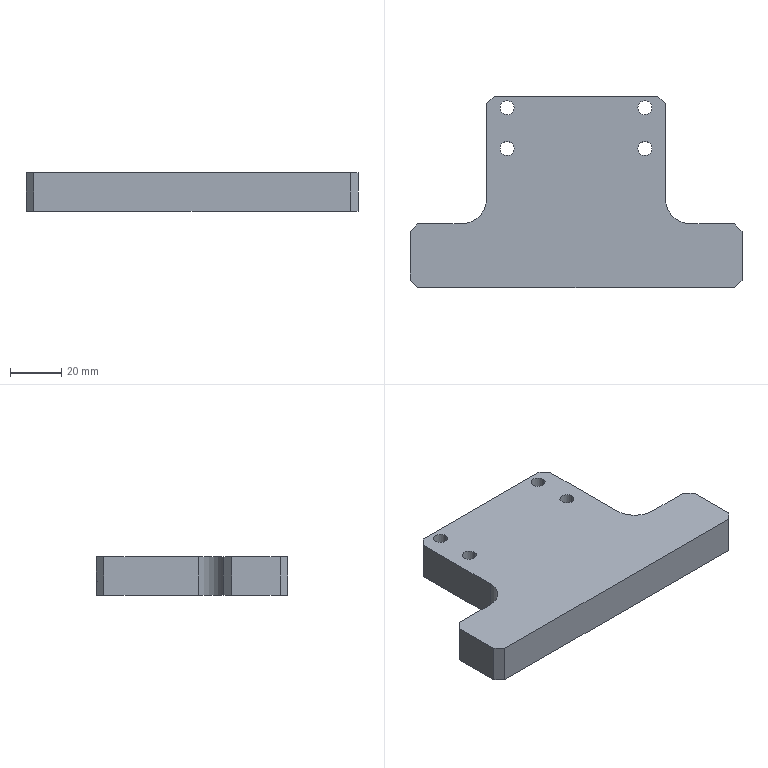Part | SolidWorks | features BaseBody 1 | 1 solid | 40 faces | box 130 x 75 x 15 mm | volume 98795 mm3 | plane 24 | cylinder 16 | commonest cylinder face diameters 5.5 x8 10 x6 20 x2
STEP:
#1=CARTESIAN_POINT('',(29.75,33.,15.));
#2=VERTEX_POINT('',#1);
#3=CARTESIAN_POINT('',(24.25,33.,15.));
#4=VERTEX_POINT('',#3);
#5=CARTESIAN_POINT('',(27.,33.,15.));
#6=DIRECTION('',(0.,0.,-1.));
#7=DIRECTION('',(-1.,0.,0.));
#8=AXIS2_PLACEMENT_3D('',#5,#6,#7);
#9=CIRCLE('',#8,2.75);
#10=EDGE_CURVE('',#2,#4,#9,.T.);
#11=ORIENTED_EDGE('',*,*,#10,.F.);
#12=CARTESIAN_POINT('',(29.75,33.,5.5));
#13=VERTEX_POINT('',#12);
#14=CARTESIAN_POINT('',(29.75,33.,0.));
#15=DIRECTION('',(0.,0.,-1.));
#16=VECTOR('',#15,1000.);
#17=LINE('',#14,#16);
#18=EDGE_CURVE('',#2,#13,#17,.T.);
#19=ORIENTED_EDGE('',*,*,#18,.T.);
#20=CARTESIAN_POINT('',(24.25,33.,5.5));
#21=VERTEX_POINT('',#20);
#22=CARTESIAN_POINT('',(27.,33.,5.5));
#23=DIRECTION('',(0.,0.,-1.));
#24=DIRECTION('',(-1.,0.,0.));
#25=AXIS2_PLACEMENT_3D('',#22,#23,#24);
#26=CIRCLE('',#25,2.75);
#27=EDGE_CURVE('',#13,#21,#26,.T.);
#28=ORIENTED_EDGE('',*,*,#27,.T.);
#29=CARTESIAN_POINT('',(24.25,33.,0.));
#30=DIRECTION('',(0.,0.,-1.));
#31=VECTOR('',#30,1000.);
#32=LINE('',#29,#31);
#33=EDGE_CURVE('',#4,#21,#32,.T.);
#34=ORIENTED_EDGE('',*,*,#33,.F.);
#35=EDGE_LOOP('',(#11,#19,#28,#34));
#36=FACE_OUTER_BOUND('',#35,.T.);
#37=CARTESIAN_POINT('',(27.,33.,0.));
#38=DIRECTION('',(0.,0.,-1.));
#39=DIRECTION('',(-1.,0.,0.));
#40=AXIS2_PLACEMENT_3D('',#37,#38,#39);
#41=CYLINDRICAL_SURFACE('',#40,2.75);
#42=ADVANCED_FACE('',(#36),#41,.F.);
#43=CARTESIAN_POINT('',(32.,17.,5.5));
#44=VERTEX_POINT('',#43);
#45=CARTESIAN_POINT('',(22.,17.,5.5));
#46=VERTEX_POINT('',#45);
#47=CARTESIAN_POINT('',(27.,17.,5.5));
#48=DIRECTION('',(0.,0.,-1.));
#49=DIRECTION('',(-1.,0.,0.));
#50=AXIS2_PLACEMENT_3D('',#47,#48,#49);
#51=CIRCLE('',#50,5.);
#52=EDGE_CURVE('',#44,#46,#51,.T.);
#53=ORIENTED_EDGE('',*,*,#52,.F.);
#54=CARTESIAN_POINT('',(32.,17.,0.));
#55=VERTEX_POINT('',#54);
#56=CARTESIAN_POINT('',(32.,17.,0.));
#57=DIRECTION('',(0.,0.,-1.));
#58=VECTOR('',#57,1000.);
#59=LINE('',#56,#58);
#60=EDGE_CURVE('',#44,#55,#59,.T.);
#61=ORIENTED_EDGE('',*,*,#60,.T.);
#62=CARTESIAN_POINT('',(22.,17.,0.));
#63=VERTEX_POINT('',#62);
#64=CARTESIAN_POINT('',(27.,17.,0.));
#65=DIRECTION('',(0.,0.,-1.));
#66=DIRECTION('',(-1.,0.,0.));
#67=AXIS2_PLACEMENT_3D('',#64,#65,#66);
#68=CIRCLE('',#67,5.);
#69=EDGE_CURVE('',#55,#63,#68,.T.);
#70=ORIENTED_EDGE('',*,*,#69,.T.);
#71=CARTESIAN_POINT('',(22.,17.,0.));
#72=DIRECTION('',(0.,0.,-1.));
#73=VECTOR('',#72,1000.);
#74=LINE('',#71,#73);
#75=EDGE_CURVE('',#46,#63,#74,.T.);
#76=ORIENTED_EDGE('',*,*,#75,.F.);
#77=EDGE_LOOP('',(#53,#61,#70,#76));
#78=FACE_OUTER_BOUND('',#77,.T.);
#79=CARTESIAN_POINT('',(27.,17.,0.));
#80=DIRECTION('',(0.,0.,-1.));
#81=DIRECTION('',(-1.,0.,0.));
#82=AXIS2_PLACEMENT_3D('',#79,#80,#81);
#83=CYLINDRICAL_SURFACE('',#82,5.);
#84=ADVANCED_FACE('',(#78),#83,.F.);
#85=CARTESIAN_POINT('',(29.75,17.,15.));
#86=VERTEX_POINT('',#85);
#87=CARTESIAN_POINT('',(24.25,17.,15.));
#88=VERTEX_POINT('',#87);
#89=CARTESIAN_POINT('',(27.,17.,15.));
#90=DIRECTION('',(0.,0.,-1.));
#91=DIRECTION('',(-1.,0.,0.));
#92=AXIS2_PLACEMENT_3D('',#89,#90,#91);
#93=CIRCLE('',#92,2.75);
#94=EDGE_CURVE('',#86,#88,#93,.T.);
#95=ORIENTED_EDGE('',*,*,#94,.F.);
#96=CARTESIAN_POINT('',(29.75,17.,5.5));
#97=VERTEX_POINT('',#96);
#98=CARTESIAN_POINT('',(29.75,17.,0.));
#99=DIRECTION('',(0.,0.,-1.));
#100=VECTOR('',#99,1000.);
#101=LINE('',#98,#100);
#102=EDGE_CURVE('',#86,#97,#101,.T.);
#103=ORIENTED_EDGE('',*,*,#102,.T.);
#104=CARTESIAN_POINT('',(24.25,17.,5.5));
#105=VERTEX_POINT('',#104);
#106=CARTESIAN_POINT('',(27.,17.,5.5));
#107=DIRECTION('',(0.,0.,-1.));
#108=DIRECTION('',(-1.,0.,0.));
#109=AXIS2_PLACEMENT_3D('',#106,#107,#108);
#110=CIRCLE('',#109,2.75);
#111=EDGE_CURVE('',#97,#105,#110,.T.);
#112=ORIENTED_EDGE('',*,*,#111,.T.);
#113=CARTESIAN_POINT('',(24.25,17.,0.));
#114=DIRECTION('',(0.,0.,-1.));
#115=VECTOR('',#114,1000.);
#116=LINE('',#113,#115);
#117=EDGE_CURVE('',#88,#105,#116,.T.);
#118=ORIENTED_EDGE('',*,*,#117,.F.);
#119=EDGE_LOOP('',(#95,#103,#112,#118));
#120=FACE_OUTER_BOUND('',#119,.T.);
#121=CARTESIAN_POINT('',(27.,17.,0.));
#122=DIRECTION('',(0.,0.,-1.));
#123=DIRECTION('',(-1.,0.,0.));
#124=AXIS2_PLACEMENT_3D('',#121,#122,#123);
#125=CYLINDRICAL_SURFACE('',#124,2.75);
#126=ADVANCED_FACE('',(#120),#125,.F.);
#127=CARTESIAN_POINT('',(-24.25,33.,15.));
#128=VERTEX_POINT('',#127);
#129=CARTESIAN_POINT('',(-29.75,33.,15.));
#130=VERTEX_POINT('',#129);
#131=CARTESIAN_POINT('',(-27.,33.,15.));
#132=DIRECTION('',(0.,0.,-1.));
#133=DIRECTION('',(-1.,0.,0.));
#134=AXIS2_PLACEMENT_3D('',#131,#132,#133);
#135=CIRCLE('',#134,2.75);
#136=EDGE_CURVE('',#128,#130,#135,.T.);
#137=ORIENTED_EDGE('',*,*,#136,.F.);
#138=CARTESIAN_POINT('',(-24.25,33.,5.5));
#139=VERTEX_POINT('',#138);
#140=CARTESIAN_POINT('',(-24.25,33.,0.));
#141=DIRECTION('',(0.,0.,-1.));
#142=VECTOR('',#141,1000.);
#143=LINE('',#140,#142);
#144=EDGE_CURVE('',#128,#139,#143,.T.);
#145=ORIENTED_EDGE('',*,*,#144,.T.);
#146=CARTESIAN_POINT('',(-29.75,33.,5.5));
#147=VERTEX_POINT('',#146);
#148=CARTESIAN_POINT('',(-27.,33.,5.5));
#149=DIRECTION('',(0.,0.,-1.));
#150=DIRECTION('',(-1.,0.,0.));
#151=AXIS2_PLACEMENT_3D('',#148,#149,#150);
#152=CIRCLE('',#151,2.75);
#153=EDGE_CURVE('',#139,#147,#152,.T.);
#154=ORIENTED_EDGE('',*,*,#153,.T.);
#155=CARTESIAN_POINT('',(-29.75,33.,0.));
#156=DIRECTION('',(0.,0.,-1.));
#157=VECTOR('',#156,1000.);
#158=LINE('',#155,#157);
#159=EDGE_CURVE('',#130,#147,#158,.T.);
#160=ORIENTED_EDGE('',*,*,#159,.F.);
#161=EDGE_LOOP('',(#137,#145,#154,#160));
#162=FACE_OUTER_BOUND('',#161,.T.);
#163=CARTESIAN_POINT('',(-27.,33.,0.));
#164=DIRECTION('',(0.,0.,-1.));
#165=DIRECTION('',(-1.,0.,0.));
#166=AXIS2_PLACEMENT_3D('',#163,#164,#165);
#167=CYLINDRICAL_SURFACE('',#166,2.75);
#168=ADVANCED_FACE('',(#162),#167,.F.);
#169=CARTESIAN_POINT('',(-22.,17.,5.5));
#170=VERTEX_POINT('',#169);
#171=CARTESIAN_POINT('',(-32.,17.,5.5));
#172=VERTEX_POINT('',#171);
#173=CARTESIAN_POINT('',(-27.,17.,5.5));
#174=DIRECTION('',(0.,0.,-1.));
#175=DIRECTION('',(-1.,0.,0.));
#176=AXIS2_PLACEMENT_3D('',#173,#174,#175);
#177=CIRCLE('',#176,5.);
#178=EDGE_CURVE('',#170,#172,#177,.T.);
#179=ORIENTED_EDGE('',*,*,#178,.F.);
#180=CARTESIAN_POINT('',(-22.,17.,0.));
#181=VERTEX_POINT('',#180);
#182=CARTESIAN_POINT('',(-22.,17.,0.));
#183=DIRECTION('',(0.,0.,-1.));
#184=VECTOR('',#183,1000.);
#185=LINE('',#182,#184);
#186=EDGE_CURVE('',#170,#181,#185,.T.);
#187=ORIENTED_EDGE('',*,*,#186,.T.);
#188=CARTESIAN_POINT('',(-32.,17.,0.));
#189=VERTEX_POINT('',#188);
#190=CARTESIAN_POINT('',(-27.,17.,0.));
#191=DIRECTION('',(0.,0.,-1.));
#192=DIRECTION('',(-1.,0.,0.));
#193=AXIS2_PLACEMENT_3D('',#190,#191,#192);
#194=CIRCLE('',#193,5.);
#195=EDGE_CURVE('',#181,#189,#194,.T.);
#196=ORIENTED_EDGE('',*,*,#195,.T.);
#197=CARTESIAN_POINT('',(-32.,17.,0.));
#198=DIRECTION('',(0.,0.,-1.));
#199=VECTOR('',#198,1000.);
#200=LINE('',#197,#199);
#201=EDGE_CURVE('',#172,#189,#200,.T.);
#202=ORIENTED_EDGE('',*,*,#201,.F.);
#203=EDGE_LOOP('',(#179,#187,#196,#202));
#204=FACE_OUTER_BOUND('',#203,.T.);
#205=CARTESIAN_POINT('',(-27.,17.,0.));
#206=DIRECTION('',(0.,0.,-1.));
#207=DIRECTION('',(-1.,0.,0.));
#208=AXIS2_PLACEMENT_3D('',#205,#206,#207);
#209=CYLINDRICAL_SURFACE('',#208,5.);
#210=ADVANCED_FACE('',(#204),#209,.F.);
#211=CARTESIAN_POINT('',(-24.25,17.,15.));
#212=VERTEX_POINT('',#211);
#213=CARTESIAN_POINT('',(-29.75,17.,15.));
#214=VERTEX_POINT('',#213);
#215=CARTESIAN_POINT('',(-27.,17.,15.));
#216=DIRECTION('',(0.,0.,-1.));
#217=DIRECTION('',(-1.,0.,0.));
#218=AXIS2_PLACEMENT_3D('',#215,#216,#217);
#219=CIRCLE('',#218,2.75);
#220=EDGE_CURVE('',#212,#214,#219,.T.);
#221=ORIENTED_EDGE('',*,*,#220,.F.);
#222=CARTESIAN_POINT('',(-24.25,17.,5.5));
#223=VERTEX_POINT('',#222);
#224=CARTESIAN_POINT('',(-24.25,17.,0.));
#225=DIRECTION('',(0.,0.,-1.));
#226=VECTOR('',#225,1000.);
#227=LINE('',#224,#226);
#228=EDGE_CURVE('',#212,#223,#227,.T.);
#229=ORIENTED_EDGE('',*,*,#228,.T.);
#230=CARTESIAN_POINT('',(-29.75,17.,5.5));
#231=VERTEX_POINT('',#230);
#232=CARTESIAN_POINT('',(-27.,17.,5.5));
#233=DIRECTION('',(0.,0.,-1.));
#234=DIRECTION('',(-1.,0.,0.));
#235=AXIS2_PLACEMENT_3D('',#232,#233,#234);
#236=CIRCLE('',#235,2.75);
#237=EDGE_CURVE('',#223,#231,#236,.T.);
#238=ORIENTED_EDGE('',*,*,#237,.T.);
#239=CARTESIAN_POINT('',(-29.75,17.,0.));
#240=DIRECTION('',(0.,0.,-1.));
#241=VECTOR('',#240,1000.);
#242=LINE('',#239,#241);
#243=EDGE_CURVE('',#214,#231,#242,.T.);
#244=ORIENTED_EDGE('',*,*,#243,.F.);
#245=EDGE_LOOP('',(#221,#229,#238,#244));
#246=FACE_OUTER_BOUND('',#245,.T.);
#247=CARTESIAN_POINT('',(-27.,17.,0.));
#248=DIRECTION('',(0.,0.,-1.));
#249=DIRECTION('',(-1.,0.,0.));
#250=AXIS2_PLACEMENT_3D('',#247,#248,#249);
#251=CYLINDRICAL_SURFACE('',#250,2.75);
#252=ADVANCED_FACE('',(#246),#251,.F.);
#253=CARTESIAN_POINT('',(32.,33.,0.));
#254=VERTEX_POINT('',#253);
#255=CARTESIAN_POINT('',(22.,33.,0.));
#256=VERTEX_POINT('',#255);
#257=CARTESIAN_POINT('',(27.,33.,0.));
#258=DIRECTION('',(0.,0.,-1.));
#259=DIRECTION('',(-1.,0.,0.));
#260=AXIS2_PLACEMENT_3D('',#257,#258,#259);
#261=CIRCLE('',#260,5.);
#262=EDGE_CURVE('',#254,#256,#261,.T.);
#263=ORIENTED_EDGE('',*,*,#262,.T.);
#264=CARTESIAN_POINT('',(22.,33.,5.5));
#265=VERTEX_POINT('',#264);
#266=CARTESIAN_POINT('',(22.,33.,27.861));
#267=DIRECTION('',(0.,0.,-1.));
#268=VECTOR('',#267,1000.);
#269=LINE('',#266,#268);
#270=EDGE_CURVE('',#265,#256,#269,.T.);
#271=ORIENTED_EDGE('',*,*,#270,.F.);
#272=CARTESIAN_POINT('',(32.,33.,5.5));
#273=VERTEX_POINT('',#272);
#274=CARTESIAN_POINT('',(27.,33.,5.5));
#275=DIRECTION('',(0.,0.,-1.));
#276=DIRECTION('',(-1.,0.,0.));
#277=AXIS2_PLACEMENT_3D('',#274,#275,#276);
#278=CIRCLE('',#277,5.);
#279=EDGE_CURVE('',#273,#265,#278,.T.);
#280=ORIENTED_EDGE('',*,*,#279,.F.);
#281=CARTESIAN_POINT('',(32.,33.,27.861));
#282=DIRECTION('',(0.,0.,-1.));
#283=VECTOR('',#282,1000.);
#284=LINE('',#281,#283);
#285=EDGE_CURVE('',#273,#254,#284,.T.);
#286=ORIENTED_EDGE('',*,*,#285,.T.);
#287=EDGE_LOOP('',(#263,#271,#280,#286));
#288=FACE_OUTER_BOUND('',#287,.T.);
#289=CARTESIAN_POINT('',(27.,33.,0.));
#290=DIRECTION('',(0.,0.,-1.));
#291=DIRECTION('',(-1.,0.,0.));
#292=AXIS2_PLACEMENT_3D('',#289,#290,#291);
#293=CYLINDRICAL_SURFACE('',#292,5.);
#294=ADVANCED_FACE('',(#288),#293,.F.);
#295=CARTESIAN_POINT('',(-22.,33.,0.));
#296=VERTEX_POINT('',#295);
#297=CARTESIAN_POINT('',(-32.,33.,0.));
#298=VERTEX_POINT('',#297);
#299=CARTESIAN_POINT('',(-27.,33.,0.));
#300=DIRECTION('',(0.,0.,-1.));
#301=DIRECTION('',(-1.,0.,0.));
#302=AXIS2_PLACEMENT_3D('',#299,#300,#301);
#303=CIRCLE('',#302,5.);
#304=EDGE_CURVE('',#296,#298,#303,.T.);
#305=ORIENTED_EDGE('',*,*,#304,.T.);
#306=CARTESIAN_POINT('',(-32.,33.,5.5));
#307=VERTEX_POINT('',#306);
#308=CARTESIAN_POINT('',(-32.,33.,27.861));
#309=DIRECTION('',(0.,0.,-1.));
#310=VECTOR('',#309,1000.);
#311=LINE('',#308,#310);
#312=EDGE_CURVE('',#307,#298,#311,.T.);
#313=ORIENTED_EDGE('',*,*,#312,.F.);
#314=CARTESIAN_POINT('',(-22.,33.,5.5));
#315=VERTEX_POINT('',#314);
#316=CARTESIAN_POINT('',(-27.,33.,5.5));
#317=DIRECTION('',(0.,0.,-1.));
#318=DIRECTION('',(-1.,0.,0.));
#319=AXIS2_PLACEMENT_3D('',#316,#317,#318);
#320=CIRCLE('',#319,5.);
#321=EDGE_CURVE('',#315,#307,#320,.T.);
#322=ORIENTED_EDGE('',*,*,#321,.F.);
#323=CARTESIAN_POINT('',(-22.,33.,27.861));
#324=DIRECTION('',(0.,0.,-1.));
#325=VECTOR('',#324,1000.);
#326=LINE('',#323,#325);
#327=EDGE_CURVE('',#315,#296,#326,.T.);
#328=ORIENTED_EDGE('',*,*,#327,.T.);
#329=EDGE_LOOP('',(#305,#313,#322,#328));
#330=FACE_OUTER_BOUND('',#329,.T.);
#331=CARTESIAN_POINT('',(-27.,33.,0.));
#332=DIRECTION('',(0.,0.,-1.));
#333=DIRECTION('',(-1.,0.,0.));
#334=AXIS2_PLACEMENT_3D('',#331,#332,#333);
#335=CYLINDRICAL_SURFACE('',#334,5.);
#336=ADVANCED_FACE('',(#330),#335,.F.);
#337=CARTESIAN_POINT('',(-65.,-15.5,15.));
#338=VERTEX_POINT('',#337);
#339=CARTESIAN_POINT('',(-65.,-34.5,15.));
#340=VERTEX_POINT('',#339);
#341=CARTESIAN_POINT('',(-65.,37.5,15.));
#342=DIRECTION('',(0.,-1.,0.));
#343=VECTOR('',#342,1000.);
#344=LINE('',#341,#343);
#345=EDGE_CURVE('',#338,#340,#344,.T.);
#346=ORIENTED_EDGE('',*,*,#345,.F.);
#347=CARTESIAN_POINT('',(-65.,-15.5,0.));
#348=VERTEX_POINT('',#347);
#349=CARTESIAN_POINT('',(-65.,-15.5,15.));
#350=DIRECTION('',(0.,0.,-1.));
#351=VECTOR('',#350,1000.);
#352=LINE('',#349,#351);
#353=EDGE_CURVE('',#338,#348,#352,.T.);
#354=ORIENTED_EDGE('',*,*,#353,.T.);
#355=CARTESIAN_POINT('',(-65.,-34.5,0.));
#356=VERTEX_POINT('',#355);
#357=CARTESIAN_POINT('',(-65.,37.5,0.));
#358=DIRECTION('',(0.,-1.,0.));
#359=VECTOR('',#358,1000.);
#360=LINE('',#357,#359);
#361=EDGE_CURVE('',#348,#356,#360,.T.);
#362=ORIENTED_EDGE('',*,*,#361,.T.);
#363=CARTESIAN_POINT('',(-65.,-34.5,15.));
#364=DIRECTION('',(0.,0.,1.));
#365=VECTOR('',#364,1000.);
#366=LINE('',#363,#365);
#367=EDGE_CURVE('',#356,#340,#366,.T.);
#368=ORIENTED_EDGE('',*,*,#367,.T.);
#369=EDGE_LOOP('',(#346,#354,#362,#368));
#370=FACE_OUTER_BOUND('',#369,.T.);
#371=CARTESIAN_POINT('',(-65.,37.5,15.));
#372=DIRECTION('',(1.,0.,0.));
#373=DIRECTION('',(0.,1.,0.));
#374=AXIS2_PLACEMENT_3D('',#371,#372,#373);
#375=PLANE('',#374);
#376=ADVANCED_FACE('',(#370),#375,.F.);
#377=CARTESIAN_POINT('',(-62.,-37.5,0.));
#378=VERTEX_POINT('',#377);
#379=CARTESIAN_POINT('',(62.,-37.5,0.));
#380=VERTEX_POINT('',#379);
#381=CARTESIAN_POINT('',(65.,-37.5,0.));
#382=DIRECTION('',(1.,0.,0.));
#383=VECTOR('',#382,1000.);
#384=LINE('',#381,#383);
#385=EDGE_CURVE('',#378,#380,#384,.T.);
#386=ORIENTED_EDGE('',*,*,#385,.T.);
#387=CARTESIAN_POINT('',(62.,-37.5,15.));
#388=VERTEX_POINT('',#387);
#389=CARTESIAN_POINT('',(62.,-37.5,15.));
#390=DIRECTION('',(0.,0.,1.));
#391=VECTOR('',#390,1000.);
#392=LINE('',#389,#391);
#393=EDGE_CURVE('',#380,#388,#392,.T.);
#394=ORIENTED_EDGE('',*,*,#393,.T.);
#395=CARTESIAN_POINT('',(-62.,-37.5,15.));
#396=VERTEX_POINT('',#395);
#397=CARTESIAN_POINT('',(65.,-37.5,15.));
#398=DIRECTION('',(1.,0.,0.));
#399=VECTOR('',#398,1000.);
#400=LINE('',#397,#399);
#401=EDGE_CURVE('',#396,#388,#400,.T.);
#402=ORIENTED_EDGE('',*,*,#401,.F.);
#403=CARTESIAN_POINT('',(-62.,-37.5,15.));
#404=DIRECTION('',(0.,0.,-1.));
#405=VECTOR('',#404,1000.);
#406=LINE('',#403,#405);
#407=EDGE_CURVE('',#396,#378,#406,.T.);
#408=ORIENTED_EDGE('',*,*,#407,.T.);
#409=EDGE_LOOP('',(#386,#394,#402,#408));
#410=FACE_OUTER_BOUND('',#409,.T.);
#411=CARTESIAN_POINT('',(65.,-37.5,15.));
#412=DIRECTION('',(0.,1.,0.));
#413=DIRECTION('',(-1.,0.,0.));
#414=AXIS2_PLACEMENT_3D('',#411,#412,#413);
#415=PLANE('',#414);
#416=ADVANCED_FACE('',(#410),#415,.F.);
#417=CARTESIAN_POINT('',(65.,-34.5,0.));
#418=VERTEX_POINT('',#417);
#419=CARTESIAN_POINT('',(65.,-15.5,0.));
#420=VERTEX_POINT('',#419);
#421=CARTESIAN_POINT('',(65.,37.5,0.));
#422=DIRECTION('',(0.,1.,0.));
#423=VECTOR('',#422,1000.);
#424=LINE('',#421,#423);
#425=EDGE_CURVE('',#418,#420,#424,.T.);
#426=ORIENTED_EDGE('',*,*,#425,.T.);
#427=CARTESIAN_POINT('',(65.,-15.5,15.));
#428=VERTEX_POINT('',#427);
#429=CARTESIAN_POINT('',(65.,-15.5,15.));
#430=DIRECTION('',(0.,0.,1.));
#431=VECTOR('',#430,1000.);
#432=LINE('',#429,#431);
#433=EDGE_CURVE('',#420,#428,#432,.T.);
#434=ORIENTED_EDGE('',*,*,#433,.T.);
#435=CARTESIAN_POINT('',(65.,-34.5,15.));
#436=VERTEX_POINT('',#435);
#437=CARTESIAN_POINT('',(65.,37.5,15.));
#438=DIRECTION('',(0.,1.,0.));
#439=VECTOR('',#438,1000.);
#440=LINE('',#437,#439);
#441=EDGE_CURVE('',#436,#428,#440,.T.);
#442=ORIENTED_EDGE('',*,*,#441,.F.);
#443=CARTESIAN_POINT('',(65.,-34.5,15.));
#444=DIRECTION('',(0.,0.,-1.));
#445=VECTOR('',#444,1000.);
#446=LINE('',#443,#445);
#447=EDGE_CURVE('',#436,#418,#446,.T.);
#448=ORIENTED_EDGE('',*,*,#447,.T.);
#449=EDGE_LOOP('',(#426,#434,#442,#448));
#450=FACE_OUTER_BOUND('',#449,.T.);
#451=CARTESIAN_POINT('',(65.,37.5,15.));
#452=DIRECTION('',(-1.,0.,0.));
#453=DIRECTION('',(0.,-1.,0.));
#454=AXIS2_PLACEMENT_3D('',#451,#452,#453);
#455=PLANE('',#454);
#456=ADVANCED_FACE('',(#450),#455,.F.);
#457=CARTESIAN_POINT('',(32.,37.5,15.));
#458=VERTEX_POINT('',#457);
#459=CARTESIAN_POINT('',(32.,37.5,5.5));
#460=VERTEX_POINT('',#459);
#461=CARTESIAN_POINT('',(32.,37.5,15.));
#462=DIRECTION('',(0.,0.,-1.));
#463=VECTOR('',#462,1000.);
#464=LINE('',#461,#463);
#465=EDGE_CURVE('',#458,#460,#464,.T.);
#466=ORIENTED_EDGE('',*,*,#465,.T.);
#467=CARTESIAN_POINT('',(22.,37.5,5.5));
#468=VERTEX_POINT('',#467);
#469=CARTESIAN_POINT('',(65.,37.5,5.5));
#470=DIRECTION('',(-1.,0.,0.));
#471=VECTOR('',#470,1000.);
#472=LINE('',#469,#471);
#473=EDGE_CURVE('',#460,#468,#472,.T.);
#474=ORIENTED_EDGE('',*,*,#473,.T.);
#475=CARTESIAN_POINT('',(22.,37.5,0.));
#476=VERTEX_POINT('',#475);
#477=CARTESIAN_POINT('',(22.,37.5,15.));
#478=DIRECTION('',(0.,0.,-1.));
#479=VECTOR('',#478,1000.);
#480=LINE('',#477,#479);
#481=EDGE_CURVE('',#468,#476,#480,.T.);
#482=ORIENTED_EDGE('',*,*,#481,.T.);
#483=CARTESIAN_POINT('',(-22.,37.5,0.));
#484=VERTEX_POINT('',#483);
#485=CARTESIAN_POINT('',(65.,37.5,0.));
#486=DIRECTION('',(-1.,0.,0.));
#487=VECTOR('',#486,1000.);
#488=LINE('',#485,#487);
#489=EDGE_CURVE('',#476,#484,#488,.T.);
#490=ORIENTED_EDGE('',*,*,#489,.T.);
#491=CARTESIAN_POINT('',(-22.,37.5,5.5));
#492=VERTEX_POINT('',#491);
#493=CARTESIAN_POINT('',(-22.,37.5,15.));
#494=DIRECTION('',(0.,0.,1.));
#495=VECTOR('',#494,1000.);
#496=LINE('',#493,#495);
#497=EDGE_CURVE('',#484,#492,#496,.T.);
#498=ORIENTED_EDGE('',*,*,#497,.T.);
#499=CARTESIAN_POINT('',(-32.,37.5,5.5));
#500=VERTEX_POINT('',#499);
#501=CARTESIAN_POINT('',(65.,37.5,5.5));
#502=DIRECTION('',(-1.,0.,0.));
#503=VECTOR('',#502,1000.);
#504=LINE('',#501,#503);
#505=EDGE_CURVE('',#492,#500,#504,.T.);
#506=ORIENTED_EDGE('',*,*,#505,.T.);
#507=CARTESIAN_POINT('',(-32.,37.5,15.));
#508=VERTEX_POINT('',#507);
#509=CARTESIAN_POINT('',(-32.,37.5,15.));
#510=DIRECTION('',(0.,0.,1.));
#511=VECTOR('',#510,1000.);
#512=LINE('',#509,#511);
#513=EDGE_CURVE('',#500,#508,#512,.T.);
#514=ORIENTED_EDGE('',*,*,#513,.T.);
#515=CARTESIAN_POINT('',(65.,37.5,15.));
#516=DIRECTION('',(-1.,0.,0.));
#517=VECTOR('',#516,1000.);
#518=LINE('',#515,#517);
#519=EDGE_CURVE('',#458,#508,#518,.T.);
#520=ORIENTED_EDGE('',*,*,#519,.F.);
#521=EDGE_LOOP('',(#466,#474,#482,#490,#498,#506,#514,#520));
#522=FACE_OUTER_BOUND('',#521,.T.);
#523=CARTESIAN_POINT('',(65.,37.5,15.));
#524=DIRECTION('',(0.,-1.,0.));
#525=DIRECTION('',(1.,0.,0.));
#526=AXIS2_PLACEMENT_3D('',#523,#524,#525);
#527=PLANE('',#526);
#528=ADVANCED_FACE('',(#522),#527,.F.);
#529=CARTESIAN_POINT('',(27.,33.,15.));
#530=DIRECTION('',(0.,0.,-1.));
#531=DIRECTION('',(-1.,0.,0.));
#532=AXIS2_PLACEMENT_3D('',#529,#530,#531);
#533=CIRCLE('',#532,2.75);
#534=EDGE_CURVE('',#4,#2,#533,.T.);
#535=ORIENTED_EDGE('',*,*,#534,.T.);
#536=ORIENTED_EDGE('',*,*,#10,.T.);
#537=EDGE_LOOP('',(#535,#536));
#538=FACE_BOUND('',#537,.T.);
#539=CARTESIAN_POINT('',(27.,17.,15.));
#540=DIRECTION('',(0.,0.,-1.));
#541=DIRECTION('',(-1.,0.,0.));
#542=AXIS2_PLACEMENT_3D('',#539,#540,#541);
#543=CIRCLE('',#542,2.75);
#544=EDGE_CURVE('',#88,#86,#543,.T.);
#545=ORIENTED_EDGE('',*,*,#544,.T.);
#546=ORIENTED_EDGE('',*,*,#94,.T.);
#547=EDGE_LOOP('',(#545,#546));
#548=FACE_BOUND('',#547,.T.);
#549=CARTESIAN_POINT('',(-27.,33.,15.));
#550=DIRECTION('',(0.,0.,-1.));
#551=DIRECTION('',(-1.,0.,0.));
#552=AXIS2_PLACEMENT_3D('',#549,#550,#551);
#553=CIRCLE('',#552,2.75);
#554=EDGE_CURVE('',#130,#128,#553,.T.);
#555=ORIENTED_EDGE('',*,*,#554,.T.);
#556=ORIENTED_EDGE('',*,*,#136,.T.);
#557=EDGE_LOOP('',(#555,#556));
#558=FACE_BOUND('',#557,.T.);
#559=CARTESIAN_POINT('',(-27.,17.,15.));
#560=DIRECTION('',(0.,0.,-1.));
#561=DIRECTION('',(-1.,0.,0.));
#562=AXIS2_PLACEMENT_3D('',#559,#560,#561);
#563=CIRCLE('',#562,2.75);
#564=EDGE_CURVE('',#214,#212,#563,.T.);
#565=ORIENTED_EDGE('',*,*,#564,.T.);
#566=ORIENTED_EDGE('',*,*,#220,.T.);
#567=EDGE_LOOP('',(#565,#566));
#568=FACE_BOUND('',#567,.T.);
#569=CARTESIAN_POINT('',(35.,-2.5,15.));
#570=VERTEX_POINT('',#569);
#571=CARTESIAN_POINT('',(35.,34.5,15.));
#572=VERTEX_POINT('',#571);
#573=CARTESIAN_POINT('',(35.,37.5,15.));
#574=DIRECTION('',(0.,1.,0.));
#575=VECTOR('',#574,1000.);
#576=LINE('',#573,#575);
#577=EDGE_CURVE('',#570,#572,#576,.T.);
#578=ORIENTED_EDGE('',*,*,#577,.T.);
#579=CARTESIAN_POINT('',(32.,37.5,15.));
#580=DIRECTION('',(-0.7071,0.7071,0.));
#581=VECTOR('',#580,1000.);
#582=LINE('',#579,#581);
#583=EDGE_CURVE('',#572,#458,#582,.T.);
#584=ORIENTED_EDGE('',*,*,#583,.T.);
#585=ORIENTED_EDGE('',*,*,#519,.T.);
#586=CARTESIAN_POINT('',(-35.,34.5,15.));
#587=VERTEX_POINT('',#586);
#588=CARTESIAN_POINT('',(-35.,34.5,15.));
#589=DIRECTION('',(-0.7071,-0.7071,0.));
#590=VECTOR('',#589,1000.);
#591=LINE('',#588,#590);
#592=EDGE_CURVE('',#508,#587,#591,.T.);
#593=ORIENTED_EDGE('',*,*,#592,.T.);
#594=CARTESIAN_POINT('',(-35.,-2.5,15.));
#595=VERTEX_POINT('',#594);
#596=CARTESIAN_POINT('',(-35.,37.5,15.));
#597=DIRECTION('',(0.,-1.,0.));
#598=VECTOR('',#597,1000.);
#599=LINE('',#596,#598);
#600=EDGE_CURVE('',#587,#595,#599,.T.);
#601=ORIENTED_EDGE('',*,*,#600,.T.);
#602=CARTESIAN_POINT('',(-45.,-12.5,15.));
#603=VERTEX_POINT('',#602);
#604=CARTESIAN_POINT('',(-45.,-2.5,15.));
#605=DIRECTION('',(0.,0.,-1.));
#606=DIRECTION('',(-1.,0.,0.));
#607=AXIS2_PLACEMENT_3D('',#604,#605,#606);
#608=CIRCLE('',#607,10.);
#609=EDGE_CURVE('',#595,#603,#608,.T.);
#610=ORIENTED_EDGE('',*,*,#609,.T.);
#611=CARTESIAN_POINT('',(-62.,-12.5,15.));
#612=VERTEX_POINT('',#611);
#613=CARTESIAN_POINT('',(-65.,-12.5,15.));
#614=DIRECTION('',(-1.,0.,0.));
#615=VECTOR('',#614,1000.);
#616=LINE('',#613,#615);
#617=EDGE_CURVE('',#603,#612,#616,.T.);
#618=ORIENTED_EDGE('',*,*,#617,.T.);
#619=CARTESIAN_POINT('',(-65.,-15.5,15.));
#620=DIRECTION('',(-0.7071,-0.7071,0.));
#621=VECTOR('',#620,1000.);
#622=LINE('',#619,#621);
#623=EDGE_CURVE('',#612,#338,#622,.T.);
#624=ORIENTED_EDGE('',*,*,#623,.T.);
#625=ORIENTED_EDGE('',*,*,#345,.T.);
#626=CARTESIAN_POINT('',(-62.,-37.5,15.));
#627=DIRECTION('',(0.7071,-0.7071,0.));
#628=VECTOR('',#627,1000.);
#629=LINE('',#626,#628);
#630=EDGE_CURVE('',#340,#396,#629,.T.);
#631=ORIENTED_EDGE('',*,*,#630,.T.);
#632=ORIENTED_EDGE('',*,*,#401,.T.);
#633=CARTESIAN_POINT('',(65.,-34.5,15.));
#634=DIRECTION('',(0.7071,0.7071,0.));
#635=VECTOR('',#634,1000.);
#636=LINE('',#633,#635);
#637=EDGE_CURVE('',#388,#436,#636,.T.);
#638=ORIENTED_EDGE('',*,*,#637,.T.);
#639=ORIENTED_EDGE('',*,*,#441,.T.);
#640=CARTESIAN_POINT('',(62.,-12.5,15.));
#641=VERTEX_POINT('',#640);
#642=CARTESIAN_POINT('',(62.,-12.5,15.));
#643=DIRECTION('',(-0.7071,0.7071,0.));
#644=VECTOR('',#643,1000.);
#645=LINE('',#642,#644);
#646=EDGE_CURVE('',#428,#641,#645,.T.);
#647=ORIENTED_EDGE('',*,*,#646,.T.);
#648=CARTESIAN_POINT('',(45.,-12.5,15.));
#649=VERTEX_POINT('',#648);
#650=CARTESIAN_POINT('',(65.,-12.5,15.));
#651=DIRECTION('',(-1.,0.,0.));
#652=VECTOR('',#651,1000.);
#653=LINE('',#650,#652);
#654=EDGE_CURVE('',#641,#649,#653,.T.);
#655=ORIENTED_EDGE('',*,*,#654,.T.);
#656=CARTESIAN_POINT('',(45.,-2.5,15.));
#657=DIRECTION('',(0.,0.,-1.));
#658=DIRECTION('',(-1.,0.,0.));
#659=AXIS2_PLACEMENT_3D('',#656,#657,#658);
#660=CIRCLE('',#659,10.);
#661=EDGE_CURVE('',#649,#570,#660,.T.);
#662=ORIENTED_EDGE('',*,*,#661,.T.);
#663=EDGE_LOOP('',(#578,#584,#585,#593,#601,#610,#618,#624,#625,#631,#632,#638,#639,#647,#655,#662));
#664=FACE_OUTER_BOUND('',#663,.T.);
#665=CARTESIAN_POINT('',(-65.,-37.5,15.));
#666=DIRECTION('',(0.,0.,-1.));
#667=DIRECTION('',(-1.,0.,0.));
#668=AXIS2_PLACEMENT_3D('',#665,#666,#667);
#669=PLANE('',#668);
#670=ADVANCED_FACE('',(#538,#548,#558,#568,#664),#669,.F.);
#671=CARTESIAN_POINT('',(22.,33.,0.));
#672=DIRECTION('',(0.,1.,0.));
#673=VECTOR('',#672,1000.);
#674=LINE('',#671,#673);
#675=EDGE_CURVE('',#256,#476,#674,.T.);
#676=ORIENTED_EDGE('',*,*,#675,.F.);
#677=ORIENTED_EDGE('',*,*,#262,.F.);
#678=CARTESIAN_POINT('',(32.,37.5,0.));
#679=VERTEX_POINT('',#678);
#680=CARTESIAN_POINT('',(32.,33.,0.));
#681=DIRECTION('',(0.,-1.,0.));
#682=VECTOR('',#681,1000.);
#683=LINE('',#680,#682);
#684=EDGE_CURVE('',#679,#254,#683,.T.);
#685=ORIENTED_EDGE('',*,*,#684,.F.);
#686=CARTESIAN_POINT('',(35.,34.5,0.));
#687=VERTEX_POINT('',#686);
#688=CARTESIAN_POINT('',(21.,48.5,0.));
#689=DIRECTION('',(0.7071,-0.7071,0.));
#690=VECTOR('',#689,1000.);
#691=LINE('',#688,#690);
#692=EDGE_CURVE('',#679,#687,#691,.T.);
#693=ORIENTED_EDGE('',*,*,#692,.T.);
#694=CARTESIAN_POINT('',(35.,-2.5,0.));
#695=VERTEX_POINT('',#694);
#696=CARTESIAN_POINT('',(35.,37.5,0.));
#697=DIRECTION('',(0.,1.,0.));
#698=VECTOR('',#697,1000.);
#699=LINE('',#696,#698);
#700=EDGE_CURVE('',#695,#687,#699,.T.);
#701=ORIENTED_EDGE('',*,*,#700,.F.);
#702=CARTESIAN_POINT('',(45.,-12.5,0.));
#703=VERTEX_POINT('',#702);
#704=CARTESIAN_POINT('',(45.,-2.5,0.));
#705=DIRECTION('',(0.,0.,1.));
#706=DIRECTION('',(-1.,0.,0.));
#707=AXIS2_PLACEMENT_3D('',#704,#705,#706);
#708=CIRCLE('',#707,10.);
#709=EDGE_CURVE('',#695,#703,#708,.T.);
#710=ORIENTED_EDGE('',*,*,#709,.T.);
#711=CARTESIAN_POINT('',(62.,-12.5,0.));
#712=VERTEX_POINT('',#711);
#713=CARTESIAN_POINT('',(65.,-12.5,0.));
#714=DIRECTION('',(-1.,0.,0.));
#715=VECTOR('',#714,1000.);
#716=LINE('',#713,#715);
#717=EDGE_CURVE('',#712,#703,#716,.T.);
#718=ORIENTED_EDGE('',*,*,#717,.F.);
#719=CARTESIAN_POINT('',(11.,38.5,0.));
#720=DIRECTION('',(0.7071,-0.7071,0.));
#721=VECTOR('',#720,1000.);
#722=LINE('',#719,#721);
#723=EDGE_CURVE('',#712,#420,#722,.T.);
#724=ORIENTED_EDGE('',*,*,#723,.T.);
#725=ORIENTED_EDGE('',*,*,#425,.F.);
#726=CARTESIAN_POINT('',(-1.5,-101.,0.));
#727=DIRECTION('',(-0.7071,-0.7071,0.));
#728=VECTOR('',#727,1000.);
#729=LINE('',#726,#728);
#730=EDGE_CURVE('',#418,#380,#729,.T.);
#731=ORIENTED_EDGE('',*,*,#730,.T.);
#732=ORIENTED_EDGE('',*,*,#385,.F.);
#733=CARTESIAN_POINT('',(-63.5,-36.,0.));
#734=DIRECTION('',(-0.7071,0.7071,0.));
#735=VECTOR('',#734,1000.);
#736=LINE('',#733,#735);
#737=EDGE_CURVE('',#378,#356,#736,.T.);
#738=ORIENTED_EDGE('',*,*,#737,.T.);
#739=ORIENTED_EDGE('',*,*,#361,.F.);
#740=CARTESIAN_POINT('',(-62.,-12.5,0.));
#741=VERTEX_POINT('',#740);
#742=CARTESIAN_POINT('',(-76.,-26.5,0.));
#743=DIRECTION('',(0.7071,0.7071,0.));
#744=VECTOR('',#743,1000.);
#745=LINE('',#742,#744);
#746=EDGE_CURVE('',#348,#741,#745,.T.);
#747=ORIENTED_EDGE('',*,*,#746,.T.);
#748=CARTESIAN_POINT('',(-45.,-12.5,0.));
#749=VERTEX_POINT('',#748);
#750=CARTESIAN_POINT('',(-65.,-12.5,0.));
#751=DIRECTION('',(-1.,0.,0.));
#752=VECTOR('',#751,1000.);
#753=LINE('',#750,#752);
#754=EDGE_CURVE('',#749,#741,#753,.T.);
#755=ORIENTED_EDGE('',*,*,#754,.F.);
#756=CARTESIAN_POINT('',(-35.,-2.5,0.));
#757=VERTEX_POINT('',#756);
#758=CARTESIAN_POINT('',(-45.,-2.5,0.));
#759=DIRECTION('',(0.,0.,1.));
#760=DIRECTION('',(-1.,0.,0.));
#761=AXIS2_PLACEMENT_3D('',#758,#759,#760);
#762=CIRCLE('',#761,10.);
#763=EDGE_CURVE('',#749,#757,#762,.T.);
#764=ORIENTED_EDGE('',*,*,#763,.T.);
#765=CARTESIAN_POINT('',(-35.,34.5,0.));
#766=VERTEX_POINT('',#765);
#767=CARTESIAN_POINT('',(-35.,37.5,0.));
#768=DIRECTION('',(0.,-1.,0.));
#769=VECTOR('',#768,1000.);
#770=LINE('',#767,#769);
#771=EDGE_CURVE('',#766,#757,#770,.T.);
#772=ORIENTED_EDGE('',*,*,#771,.F.);
#773=CARTESIAN_POINT('',(-32.,37.5,0.));
#774=VERTEX_POINT('',#773);
#775=CARTESIAN_POINT('',(-86.,-16.5,0.));
#776=DIRECTION('',(0.7071,0.7071,0.));
#777=VECTOR('',#776,1000.);
#778=LINE('',#775,#777);
#779=EDGE_CURVE('',#766,#774,#778,.T.);
#780=ORIENTED_EDGE('',*,*,#779,.T.);
#781=CARTESIAN_POINT('',(-32.,33.,0.));
#782=DIRECTION('',(0.,1.,0.));
#783=VECTOR('',#782,1000.);
#784=LINE('',#781,#783);
#785=EDGE_CURVE('',#298,#774,#784,.T.);
#786=ORIENTED_EDGE('',*,*,#785,.F.);
#787=ORIENTED_EDGE('',*,*,#304,.F.);
#788=CARTESIAN_POINT('',(-22.,33.,0.));
#789=DIRECTION('',(0.,-1.,0.));
#790=VECTOR('',#789,1000.);
#791=LINE('',#788,#790);
#792=EDGE_CURVE('',#484,#296,#791,.T.);
#793=ORIENTED_EDGE('',*,*,#792,.F.);
#794=ORIENTED_EDGE('',*,*,#489,.F.);
#795=EDGE_LOOP('',(#676,#677,#685,#693,#701,#710,#718,#724,#725,#731,#732,#738,#739,#747,#755,#764,#772,#780,#786,#787,#793,#794));
#796=FACE_OUTER_BOUND('',#795,.T.);
#797=CARTESIAN_POINT('',(27.,17.,0.));
#798=DIRECTION('',(0.,0.,-1.));
#799=DIRECTION('',(-1.,0.,0.));
#800=AXIS2_PLACEMENT_3D('',#797,#798,#799);
#801=CIRCLE('',#800,5.);
#802=EDGE_CURVE('',#63,#55,#801,.T.);
#803=ORIENTED_EDGE('',*,*,#802,.F.);
#804=ORIENTED_EDGE('',*,*,#69,.F.);
#805=EDGE_LOOP('',(#803,#804));
#806=FACE_BOUND('',#805,.T.);
#807=CARTESIAN_POINT('',(-27.,17.,0.));
#808=DIRECTION('',(0.,0.,-1.));
#809=DIRECTION('',(-1.,0.,0.));
#810=AXIS2_PLACEMENT_3D('',#807,#808,#809);
#811=CIRCLE('',#810,5.);
#812=EDGE_CURVE('',#189,#181,#811,.T.);
#813=ORIENTED_EDGE('',*,*,#812,.F.);
#814=ORIENTED_EDGE('',*,*,#195,.F.);
#815=EDGE_LOOP('',(#813,#814));
#816=FACE_BOUND('',#815,.T.);
#817=CARTESIAN_POINT('',(-65.,-37.5,0.));
#818=DIRECTION('',(0.,0.,-1.));
#819=DIRECTION('',(-1.,0.,0.));
#820=AXIS2_PLACEMENT_3D('',#817,#818,#819);
#821=PLANE('',#820);
#822=ADVANCED_FACE('',(#796,#806,#816),#821,.T.);
#823=ORIENTED_EDGE('',*,*,#228,.F.);
#824=ORIENTED_EDGE('',*,*,#564,.F.);
#825=ORIENTED_EDGE('',*,*,#243,.T.);
#826=CARTESIAN_POINT('',(-27.,17.,5.5));
#827=DIRECTION('',(0.,0.,-1.));
#828=DIRECTION('',(-1.,0.,0.));
#829=AXIS2_PLACEMENT_3D('',#826,#827,#828);
#830=CIRCLE('',#829,2.75);
#831=EDGE_CURVE('',#231,#223,#830,.T.);
#832=ORIENTED_EDGE('',*,*,#831,.T.);
#833=EDGE_LOOP('',(#823,#824,#825,#832));
#834=FACE_OUTER_BOUND('',#833,.T.);
#835=CARTESIAN_POINT('',(-27.,17.,0.));
#836=DIRECTION('',(0.,0.,-1.));
#837=DIRECTION('',(-1.,0.,0.));
#838=AXIS2_PLACEMENT_3D('',#835,#836,#837);
#839=CYLINDRICAL_SURFACE('',#838,2.75);
#840=ADVANCED_FACE('',(#834),#839,.F.);
#841=ORIENTED_EDGE('',*,*,#831,.F.);
#842=ORIENTED_EDGE('',*,*,#237,.F.);
#843=EDGE_LOOP('',(#841,#842));
#844=FACE_BOUND('',#843,.T.);
#845=CARTESIAN_POINT('',(-27.,17.,5.5));
#846=DIRECTION('',(0.,0.,-1.));
#847=DIRECTION('',(-1.,0.,0.));
#848=AXIS2_PLACEMENT_3D('',#845,#846,#847);
#849=CIRCLE('',#848,5.);
#850=EDGE_CURVE('',#172,#170,#849,.T.);
#851=ORIENTED_EDGE('',*,*,#850,.T.);
#852=ORIENTED_EDGE('',*,*,#178,.T.);
#853=EDGE_LOOP('',(#851,#852));
#854=FACE_OUTER_BOUND('',#853,.T.);
#855=CARTESIAN_POINT('',(-24.25,17.,5.5));
#856=DIRECTION('',(0.,0.,1.));
#857=DIRECTION('',(1.,0.,0.));
#858=AXIS2_PLACEMENT_3D('',#855,#856,#857);
#859=PLANE('',#858);
#860=ADVANCED_FACE('',(#844,#854),#859,.F.);
#861=ORIENTED_EDGE('',*,*,#186,.F.);
#862=ORIENTED_EDGE('',*,*,#850,.F.);
#863=ORIENTED_EDGE('',*,*,#201,.T.);
#864=ORIENTED_EDGE('',*,*,#812,.T.);
#865=EDGE_LOOP('',(#861,#862,#863,#864));
#866=FACE_OUTER_BOUND('',#865,.T.);
#867=CARTESIAN_POINT('',(-27.,17.,0.));
#868=DIRECTION('',(0.,0.,-1.));
#869=DIRECTION('',(-1.,0.,0.));
#870=AXIS2_PLACEMENT_3D('',#867,#868,#869);
#871=CYLINDRICAL_SURFACE('',#870,5.);
#872=ADVANCED_FACE('',(#866),#871,.F.);
#873=CARTESIAN_POINT('',(-27.,33.,5.5));
#874=DIRECTION('',(0.,0.,-1.));
#875=DIRECTION('',(-1.,0.,0.));
#876=AXIS2_PLACEMENT_3D('',#873,#874,#875);
#877=CIRCLE('',#876,2.75);
#878=EDGE_CURVE('',#147,#139,#877,.T.);
#879=ORIENTED_EDGE('',*,*,#878,.F.);
#880=ORIENTED_EDGE('',*,*,#153,.F.);
#881=EDGE_LOOP('',(#879,#880));
#882=FACE_BOUND('',#881,.T.);
#883=ORIENTED_EDGE('',*,*,#505,.F.);
#884=CARTESIAN_POINT('',(-22.,33.,5.5));
#885=DIRECTION('',(0.,-1.,0.));
#886=VECTOR('',#885,1000.);
#887=LINE('',#884,#886);
#888=EDGE_CURVE('',#492,#315,#887,.T.);
#889=ORIENTED_EDGE('',*,*,#888,.T.);
#890=ORIENTED_EDGE('',*,*,#321,.T.);
#891=CARTESIAN_POINT('',(-32.,33.,5.5));
#892=DIRECTION('',(0.,1.,0.));
#893=VECTOR('',#892,1000.);
#894=LINE('',#891,#893);
#895=EDGE_CURVE('',#307,#500,#894,.T.);
#896=ORIENTED_EDGE('',*,*,#895,.T.);
#897=EDGE_LOOP('',(#883,#889,#890,#896));
#898=FACE_OUTER_BOUND('',#897,.T.);
#899=CARTESIAN_POINT('',(-24.25,33.,5.5));
#900=DIRECTION('',(0.,0.,1.));
#901=DIRECTION('',(1.,0.,0.));
#902=AXIS2_PLACEMENT_3D('',#899,#900,#901);
#903=PLANE('',#902);
#904=ADVANCED_FACE('',(#882,#898),#903,.F.);
#905=ORIENTED_EDGE('',*,*,#144,.F.);
#906=ORIENTED_EDGE('',*,*,#554,.F.);
#907=ORIENTED_EDGE('',*,*,#159,.T.);
#908=ORIENTED_EDGE('',*,*,#878,.T.);
#909=EDGE_LOOP('',(#905,#906,#907,#908));
#910=FACE_OUTER_BOUND('',#909,.T.);
#911=CARTESIAN_POINT('',(-27.,33.,0.));
#912=DIRECTION('',(0.,0.,-1.));
#913=DIRECTION('',(-1.,0.,0.));
#914=AXIS2_PLACEMENT_3D('',#911,#912,#913);
#915=CYLINDRICAL_SURFACE('',#914,2.75);
#916=ADVANCED_FACE('',(#910),#915,.F.);
#917=ORIENTED_EDGE('',*,*,#102,.F.);
#918=ORIENTED_EDGE('',*,*,#544,.F.);
#919=ORIENTED_EDGE('',*,*,#117,.T.);
#920=CARTESIAN_POINT('',(27.,17.,5.5));
#921=DIRECTION('',(0.,0.,-1.));
#922=DIRECTION('',(-1.,0.,0.));
#923=AXIS2_PLACEMENT_3D('',#920,#921,#922);
#924=CIRCLE('',#923,2.75);
#925=EDGE_CURVE('',#105,#97,#924,.T.);
#926=ORIENTED_EDGE('',*,*,#925,.T.);
#927=EDGE_LOOP('',(#917,#918,#919,#926));
#928=FACE_OUTER_BOUND('',#927,.T.);
#929=CARTESIAN_POINT('',(27.,17.,0.));
#930=DIRECTION('',(0.,0.,-1.));
#931=DIRECTION('',(-1.,0.,0.));
#932=AXIS2_PLACEMENT_3D('',#929,#930,#931);
#933=CYLINDRICAL_SURFACE('',#932,2.75);
#934=ADVANCED_FACE('',(#928),#933,.F.);
#935=ORIENTED_EDGE('',*,*,#925,.F.);
#936=ORIENTED_EDGE('',*,*,#111,.F.);
#937=EDGE_LOOP('',(#935,#936));
#938=FACE_BOUND('',#937,.T.);
#939=CARTESIAN_POINT('',(27.,17.,5.5));
#940=DIRECTION('',(0.,0.,-1.));
#941=DIRECTION('',(-1.,0.,0.));
#942=AXIS2_PLACEMENT_3D('',#939,#940,#941);
#943=CIRCLE('',#942,5.);
#944=EDGE_CURVE('',#46,#44,#943,.T.);
#945=ORIENTED_EDGE('',*,*,#944,.T.);
#946=ORIENTED_EDGE('',*,*,#52,.T.);
#947=EDGE_LOOP('',(#945,#946));
#948=FACE_OUTER_BOUND('',#947,.T.);
#949=CARTESIAN_POINT('',(29.75,17.,5.5));
#950=DIRECTION('',(0.,0.,1.));
#951=DIRECTION('',(1.,0.,0.));
#952=AXIS2_PLACEMENT_3D('',#949,#950,#951);
#953=PLANE('',#952);
#954=ADVANCED_FACE('',(#938,#948),#953,.F.);
#955=ORIENTED_EDGE('',*,*,#60,.F.);
#956=ORIENTED_EDGE('',*,*,#944,.F.);
#957=ORIENTED_EDGE('',*,*,#75,.T.);
#958=ORIENTED_EDGE('',*,*,#802,.T.);
#959=EDGE_LOOP('',(#955,#956,#957,#958));
#960=FACE_OUTER_BOUND('',#959,.T.);
#961=CARTESIAN_POINT('',(27.,17.,0.));
#962=DIRECTION('',(0.,0.,-1.));
#963=DIRECTION('',(-1.,0.,0.));
#964=AXIS2_PLACEMENT_3D('',#961,#962,#963);
#965=CYLINDRICAL_SURFACE('',#964,5.);
#966=ADVANCED_FACE('',(#960),#965,.F.);
#967=CARTESIAN_POINT('',(27.,33.,5.5));
#968=DIRECTION('',(0.,0.,-1.));
#969=DIRECTION('',(-1.,0.,0.));
#970=AXIS2_PLACEMENT_3D('',#967,#968,#969);
#971=CIRCLE('',#970,2.75);
#972=EDGE_CURVE('',#21,#13,#971,.T.);
#973=ORIENTED_EDGE('',*,*,#972,.F.);
#974=ORIENTED_EDGE('',*,*,#27,.F.);
#975=EDGE_LOOP('',(#973,#974));
#976=FACE_BOUND('',#975,.T.);
#977=ORIENTED_EDGE('',*,*,#473,.F.);
#978=CARTESIAN_POINT('',(32.,33.,5.5));
#979=DIRECTION('',(0.,-1.,0.));
#980=VECTOR('',#979,1000.);
#981=LINE('',#978,#980);
#982=EDGE_CURVE('',#460,#273,#981,.T.);
#983=ORIENTED_EDGE('',*,*,#982,.T.);
#984=ORIENTED_EDGE('',*,*,#279,.T.);
#985=CARTESIAN_POINT('',(22.,33.,5.5));
#986=DIRECTION('',(0.,1.,0.));
#987=VECTOR('',#986,1000.);
#988=LINE('',#985,#987);
#989=EDGE_CURVE('',#265,#468,#988,.T.);
#990=ORIENTED_EDGE('',*,*,#989,.T.);
#991=EDGE_LOOP('',(#977,#983,#984,#990));
#992=FACE_OUTER_BOUND('',#991,.T.);
#993=CARTESIAN_POINT('',(29.75,33.,5.5));
#994=DIRECTION('',(0.,0.,1.));
#995=DIRECTION('',(1.,0.,0.));
#996=AXIS2_PLACEMENT_3D('',#993,#994,#995);
#997=PLANE('',#996);
#998=ADVANCED_FACE('',(#976,#992),#997,.F.);
#999=ORIENTED_EDGE('',*,*,#18,.F.);
#1000=ORIENTED_EDGE('',*,*,#534,.F.);
#1001=ORIENTED_EDGE('',*,*,#33,.T.);
#1002=ORIENTED_EDGE('',*,*,#972,.T.);
#1003=EDGE_LOOP('',(#999,#1000,#1001,#1002));
#1004=FACE_OUTER_BOUND('',#1003,.T.);
#1005=CARTESIAN_POINT('',(27.,33.,0.));
#1006=DIRECTION('',(0.,0.,-1.));
#1007=DIRECTION('',(-1.,0.,0.));
#1008=AXIS2_PLACEMENT_3D('',#1005,#1006,#1007);
#1009=CYLINDRICAL_SURFACE('',#1008,2.75);
#1010=ADVANCED_FACE('',(#1004),#1009,.F.);
#1011=ORIENTED_EDGE('',*,*,#754,.T.);
#1012=CARTESIAN_POINT('',(-62.,-12.5,15.));
#1013=DIRECTION('',(0.,0.,1.));
#1014=VECTOR('',#1013,1000.);
#1015=LINE('',#1012,#1014);
#1016=EDGE_CURVE('',#741,#612,#1015,.T.);
#1017=ORIENTED_EDGE('',*,*,#1016,.T.);
#1018=ORIENTED_EDGE('',*,*,#617,.F.);
#1019=CARTESIAN_POINT('',(-45.,-12.5,0.));
#1020=DIRECTION('',(0.,0.,-1.));
#1021=VECTOR('',#1020,1000.);
#1022=LINE('',#1019,#1021);
#1023=EDGE_CURVE('',#603,#749,#1022,.T.);
#1024=ORIENTED_EDGE('',*,*,#1023,.T.);
#1025=EDGE_LOOP('',(#1011,#1017,#1018,#1024));
#1026=FACE_OUTER_BOUND('',#1025,.T.);
#1027=CARTESIAN_POINT('',(-65.,-12.5,15.));
#1028=DIRECTION('',(0.,-1.,0.));
#1029=DIRECTION('',(1.,0.,0.));
#1030=AXIS2_PLACEMENT_3D('',#1027,#1028,#1029);
#1031=PLANE('',#1030);
#1032=ADVANCED_FACE('',(#1026),#1031,.F.);
#1033=ORIENTED_EDGE('',*,*,#600,.F.);
#1034=CARTESIAN_POINT('',(-35.,34.5,15.));
#1035=DIRECTION('',(0.,0.,-1.));
#1036=VECTOR('',#1035,1000.);
#1037=LINE('',#1034,#1036);
#1038=EDGE_CURVE('',#587,#766,#1037,.T.);
#1039=ORIENTED_EDGE('',*,*,#1038,.T.);
#1040=ORIENTED_EDGE('',*,*,#771,.T.);
#1041=CARTESIAN_POINT('',(-35.,-2.5,15.));
#1042=DIRECTION('',(0.,0.,1.));
#1043=VECTOR('',#1042,1000.);
#1044=LINE('',#1041,#1043);
#1045=EDGE_CURVE('',#757,#595,#1044,.T.);
#1046=ORIENTED_EDGE('',*,*,#1045,.T.);
#1047=EDGE_LOOP('',(#1033,#1039,#1040,#1046));
#1048=FACE_OUTER_BOUND('',#1047,.T.);
#1049=CARTESIAN_POINT('',(-35.,37.5,15.));
#1050=DIRECTION('',(1.,0.,0.));
#1051=DIRECTION('',(0.,1.,0.));
#1052=AXIS2_PLACEMENT_3D('',#1049,#1050,#1051);
#1053=PLANE('',#1052);
#1054=ADVANCED_FACE('',(#1048),#1053,.F.);
#1055=ORIENTED_EDGE('',*,*,#700,.T.);
#1056=CARTESIAN_POINT('',(35.,34.5,15.));
#1057=DIRECTION('',(0.,0.,1.));
#1058=VECTOR('',#1057,1000.);
#1059=LINE('',#1056,#1058);
#1060=EDGE_CURVE('',#687,#572,#1059,.T.);
#1061=ORIENTED_EDGE('',*,*,#1060,.T.);
#1062=ORIENTED_EDGE('',*,*,#577,.F.);
#1063=CARTESIAN_POINT('',(35.,-2.5,0.));
#1064=DIRECTION('',(0.,0.,-1.));
#1065=VECTOR('',#1064,1000.);
#1066=LINE('',#1063,#1065);
#1067=EDGE_CURVE('',#570,#695,#1066,.T.);
#1068=ORIENTED_EDGE('',*,*,#1067,.T.);
#1069=EDGE_LOOP('',(#1055,#1061,#1062,#1068));
#1070=FACE_OUTER_BOUND('',#1069,.T.);
#1071=CARTESIAN_POINT('',(35.,37.5,15.));
#1072=DIRECTION('',(-1.,0.,0.));
#1073=DIRECTION('',(0.,-1.,0.));
#1074=AXIS2_PLACEMENT_3D('',#1071,#1072,#1073);
#1075=PLANE('',#1074);
#1076=ADVANCED_FACE('',(#1070),#1075,.F.);
#1077=ORIENTED_EDGE('',*,*,#654,.F.);
#1078=CARTESIAN_POINT('',(62.,-12.5,15.));
#1079=DIRECTION('',(0.,0.,-1.));
#1080=VECTOR('',#1079,1000.);
#1081=LINE('',#1078,#1080);
#1082=EDGE_CURVE('',#641,#712,#1081,.T.);
#1083=ORIENTED_EDGE('',*,*,#1082,.T.);
#1084=ORIENTED_EDGE('',*,*,#717,.T.);
#1085=CARTESIAN_POINT('',(45.,-12.5,15.));
#1086=DIRECTION('',(0.,0.,1.));
#1087=VECTOR('',#1086,1000.);
#1088=LINE('',#1085,#1087);
#1089=EDGE_CURVE('',#703,#649,#1088,.T.);
#1090=ORIENTED_EDGE('',*,*,#1089,.T.);
#1091=EDGE_LOOP('',(#1077,#1083,#1084,#1090));
#1092=FACE_OUTER_BOUND('',#1091,.T.);
#1093=CARTESIAN_POINT('',(65.,-12.5,15.));
#1094=DIRECTION('',(0.,-1.,0.));
#1095=DIRECTION('',(1.,0.,0.));
#1096=AXIS2_PLACEMENT_3D('',#1093,#1094,#1095);
#1097=PLANE('',#1096);
#1098=ADVANCED_FACE('',(#1092),#1097,.F.);
#1099=ORIENTED_EDGE('',*,*,#661,.F.);
#1100=ORIENTED_EDGE('',*,*,#1089,.F.);
#1101=ORIENTED_EDGE('',*,*,#709,.F.);
#1102=ORIENTED_EDGE('',*,*,#1067,.F.);
#1103=EDGE_LOOP('',(#1099,#1100,#1101,#1102));
#1104=FACE_OUTER_BOUND('',#1103,.T.);
#1105=CARTESIAN_POINT('',(45.,-2.5,15.));
#1106=DIRECTION('',(0.,0.,1.));
#1107=DIRECTION('',(1.,0.,0.));
#1108=AXIS2_PLACEMENT_3D('',#1105,#1106,#1107);
#1109=CYLINDRICAL_SURFACE('',#1108,10.);
#1110=ADVANCED_FACE('',(#1104),#1109,.F.);
#1111=ORIENTED_EDGE('',*,*,#609,.F.);
#1112=ORIENTED_EDGE('',*,*,#1045,.F.);
#1113=ORIENTED_EDGE('',*,*,#763,.F.);
#1114=ORIENTED_EDGE('',*,*,#1023,.F.);
#1115=EDGE_LOOP('',(#1111,#1112,#1113,#1114));
#1116=FACE_OUTER_BOUND('',#1115,.T.);
#1117=CARTESIAN_POINT('',(-45.,-2.5,15.));
#1118=DIRECTION('',(0.,0.,1.));
#1119=DIRECTION('',(1.,0.,0.));
#1120=AXIS2_PLACEMENT_3D('',#1117,#1118,#1119);
#1121=CYLINDRICAL_SURFACE('',#1120,10.);
#1122=ADVANCED_FACE('',(#1116),#1121,.F.);
#1123=ORIENTED_EDGE('',*,*,#583,.F.);
#1124=ORIENTED_EDGE('',*,*,#1060,.F.);
#1125=ORIENTED_EDGE('',*,*,#692,.F.);
#1126=CARTESIAN_POINT('',(32.,37.5,15.));
#1127=DIRECTION('',(0.,0.,-1.));
#1128=VECTOR('',#1127,1000.);
#1129=LINE('',#1126,#1128);
#1130=EDGE_CURVE('',#460,#679,#1129,.T.);
#1131=ORIENTED_EDGE('',*,*,#1130,.F.);
#1132=ORIENTED_EDGE('',*,*,#465,.F.);
#1133=EDGE_LOOP('',(#1123,#1124,#1125,#1131,#1132));
#1134=FACE_OUTER_BOUND('',#1133,.T.);
#1135=CARTESIAN_POINT('',(32.,37.5,15.));
#1136=DIRECTION('',(-0.7071,-0.7071,0.));
#1137=DIRECTION('',(0.,0.,-1.));
#1138=AXIS2_PLACEMENT_3D('',#1135,#1136,#1137);
#1139=PLANE('',#1138);
#1140=ADVANCED_FACE('',(#1134),#1139,.F.);
#1141=ORIENTED_EDGE('',*,*,#592,.F.);
#1142=ORIENTED_EDGE('',*,*,#513,.F.);
#1143=CARTESIAN_POINT('',(-32.,37.5,15.));
#1144=DIRECTION('',(0.,0.,1.));
#1145=VECTOR('',#1144,1000.);
#1146=LINE('',#1143,#1145);
#1147=EDGE_CURVE('',#774,#500,#1146,.T.);
#1148=ORIENTED_EDGE('',*,*,#1147,.F.);
#1149=ORIENTED_EDGE('',*,*,#779,.F.);
#1150=ORIENTED_EDGE('',*,*,#1038,.F.);
#1151=EDGE_LOOP('',(#1141,#1142,#1148,#1149,#1150));
#1152=FACE_OUTER_BOUND('',#1151,.T.);
#1153=CARTESIAN_POINT('',(-35.,34.5,15.));
#1154=DIRECTION('',(0.7071,-0.7071,0.));
#1155=DIRECTION('',(0.,0.,-1.));
#1156=AXIS2_PLACEMENT_3D('',#1153,#1154,#1155);
#1157=PLANE('',#1156);
#1158=ADVANCED_FACE('',(#1152),#1157,.F.);
#1159=ORIENTED_EDGE('',*,*,#646,.F.);
#1160=ORIENTED_EDGE('',*,*,#433,.F.);
#1161=ORIENTED_EDGE('',*,*,#723,.F.);
#1162=ORIENTED_EDGE('',*,*,#1082,.F.);
#1163=EDGE_LOOP('',(#1159,#1160,#1161,#1162));
#1164=FACE_OUTER_BOUND('',#1163,.T.);
#1165=CARTESIAN_POINT('',(62.,-12.5,15.));
#1166=DIRECTION('',(-0.7071,-0.7071,0.));
#1167=DIRECTION('',(0.,0.,-1.));
#1168=AXIS2_PLACEMENT_3D('',#1165,#1166,#1167);
#1169=PLANE('',#1168);
#1170=ADVANCED_FACE('',(#1164),#1169,.F.);
#1171=ORIENTED_EDGE('',*,*,#637,.F.);
#1172=ORIENTED_EDGE('',*,*,#393,.F.);
#1173=ORIENTED_EDGE('',*,*,#730,.F.);
#1174=ORIENTED_EDGE('',*,*,#447,.F.);
#1175=EDGE_LOOP('',(#1171,#1172,#1173,#1174));
#1176=FACE_OUTER_BOUND('',#1175,.T.);
#1177=CARTESIAN_POINT('',(65.,-34.5,15.));
#1178=DIRECTION('',(-0.7071,0.7071,0.));
#1179=DIRECTION('',(0.,0.,-1.));
#1180=AXIS2_PLACEMENT_3D('',#1177,#1178,#1179);
#1181=PLANE('',#1180);
#1182=ADVANCED_FACE('',(#1176),#1181,.F.);
#1183=ORIENTED_EDGE('',*,*,#623,.F.);
#1184=ORIENTED_EDGE('',*,*,#1016,.F.);
#1185=ORIENTED_EDGE('',*,*,#746,.F.);
#1186=ORIENTED_EDGE('',*,*,#353,.F.);
#1187=EDGE_LOOP('',(#1183,#1184,#1185,#1186));
#1188=FACE_OUTER_BOUND('',#1187,.T.);
#1189=CARTESIAN_POINT('',(-65.,-15.5,15.));
#1190=DIRECTION('',(0.7071,-0.7071,0.));
#1191=DIRECTION('',(0.,0.,-1.));
#1192=AXIS2_PLACEMENT_3D('',#1189,#1190,#1191);
#1193=PLANE('',#1192);
#1194=ADVANCED_FACE('',(#1188),#1193,.F.);
#1195=ORIENTED_EDGE('',*,*,#630,.F.);
#1196=ORIENTED_EDGE('',*,*,#367,.F.);
#1197=ORIENTED_EDGE('',*,*,#737,.F.);
#1198=ORIENTED_EDGE('',*,*,#407,.F.);
#1199=EDGE_LOOP('',(#1195,#1196,#1197,#1198));
#1200=FACE_OUTER_BOUND('',#1199,.T.);
#1201=CARTESIAN_POINT('',(-62.,-37.5,15.));
#1202=DIRECTION('',(0.7071,0.7071,0.));
#1203=DIRECTION('',(0.,0.,-1.));
#1204=AXIS2_PLACEMENT_3D('',#1201,#1202,#1203);
#1205=PLANE('',#1204);
#1206=ADVANCED_FACE('',(#1200),#1205,.F.);
#1207=ORIENTED_EDGE('',*,*,#1147,.T.);
#1208=ORIENTED_EDGE('',*,*,#895,.F.);
#1209=ORIENTED_EDGE('',*,*,#312,.T.);
#1210=ORIENTED_EDGE('',*,*,#785,.T.);
#1211=EDGE_LOOP('',(#1207,#1208,#1209,#1210));
#1212=FACE_OUTER_BOUND('',#1211,.T.);
#1213=CARTESIAN_POINT('',(-32.,33.,27.861));
#1214=DIRECTION('',(-1.,0.,0.));
#1215=DIRECTION('',(0.,0.,1.));
#1216=AXIS2_PLACEMENT_3D('',#1213,#1214,#1215);
#1217=PLANE('',#1216);
#1218=ADVANCED_FACE('',(#1212),#1217,.F.);
#1219=ORIENTED_EDGE('',*,*,#792,.T.);
#1220=ORIENTED_EDGE('',*,*,#327,.F.);
#1221=ORIENTED_EDGE('',*,*,#888,.F.);
#1222=ORIENTED_EDGE('',*,*,#497,.F.);
#1223=EDGE_LOOP('',(#1219,#1220,#1221,#1222));
#1224=FACE_OUTER_BOUND('',#1223,.T.);
#1225=CARTESIAN_POINT('',(-22.,33.,27.861));
#1226=DIRECTION('',(1.,0.,0.));
#1227=DIRECTION('',(0.,0.,-1.));
#1228=AXIS2_PLACEMENT_3D('',#1225,#1226,#1227);
#1229=PLANE('',#1228);
#1230=ADVANCED_FACE('',(#1224),#1229,.F.);
#1231=ORIENTED_EDGE('',*,*,#1130,.T.);
#1232=ORIENTED_EDGE('',*,*,#684,.T.);
#1233=ORIENTED_EDGE('',*,*,#285,.F.);
#1234=ORIENTED_EDGE('',*,*,#982,.F.);
#1235=EDGE_LOOP('',(#1231,#1232,#1233,#1234));
#1236=FACE_OUTER_BOUND('',#1235,.T.);
#1237=CARTESIAN_POINT('',(32.,33.,27.861));
#1238=DIRECTION('',(1.,0.,0.));
#1239=DIRECTION('',(0.,0.,-1.));
#1240=AXIS2_PLACEMENT_3D('',#1237,#1238,#1239);
#1241=PLANE('',#1240);
#1242=ADVANCED_FACE('',(#1236),#1241,.F.);
#1243=ORIENTED_EDGE('',*,*,#989,.F.);
#1244=ORIENTED_EDGE('',*,*,#270,.T.);
#1245=ORIENTED_EDGE('',*,*,#675,.T.);
#1246=ORIENTED_EDGE('',*,*,#481,.F.);
#1247=EDGE_LOOP('',(#1243,#1244,#1245,#1246));
#1248=FACE_OUTER_BOUND('',#1247,.T.);
#1249=CARTESIAN_POINT('',(22.,33.,27.861));
#1250=DIRECTION('',(-1.,0.,0.));
#1251=DIRECTION('',(0.,0.,1.));
#1252=AXIS2_PLACEMENT_3D('',#1249,#1250,#1251);
#1253=PLANE('',#1252);
#1254=ADVANCED_FACE('',(#1248),#1253,.F.);
#1255=CLOSED_SHELL('',(#42,#84,#126,#168,#210,#252,#294,#336,#376,#416,#456,#528,#670,#822,#840,#860,#872,#904,#916,#934,#954,#966,#998,#1010,#1032,#1054,#1076,#1098,#1110,#1122,#1140,#1158,#1170,#1182,#1194,#1206,#1218,#1230,#1242,#1254));
#1256=MANIFOLD_SOLID_BREP('',#1255);
#1257=CARTESIAN_POINT('',(0.,0.,0.));
#1258=DIRECTION('',(0.,0.,1.));
#1259=DIRECTION('',(1.,0.,0.));
#1260=AXIS2_PLACEMENT_3D('',#1257,#1258,#1259);
#1261=(LENGTH_UNIT()NAMED_UNIT(*)SI_UNIT(.MILLI.,.METRE.));
#1262=UNCERTAINTY_MEASURE_WITH_UNIT(LENGTH_MEASURE(0.00001),#1261,'','');
#1263=(NAMED_UNIT(*)PLANE_ANGLE_UNIT()SI_UNIT($,.RADIAN.));
#1264=(NAMED_UNIT(*)SI_UNIT($,.STERADIAN.)SOLID_ANGLE_UNIT());
#1265=(GEOMETRIC_REPRESENTATION_CONTEXT(3)GLOBAL_UNCERTAINTY_ASSIGNED_CONTEXT((#1262))GLOBAL_UNIT_ASSIGNED_CONTEXT((#1261,#1263,#1264))REPRESENTATION_CONTEXT('',''));
#1266=ADVANCED_BREP_SHAPE_REPRESENTATION('',(#1256,#1260),#1265);